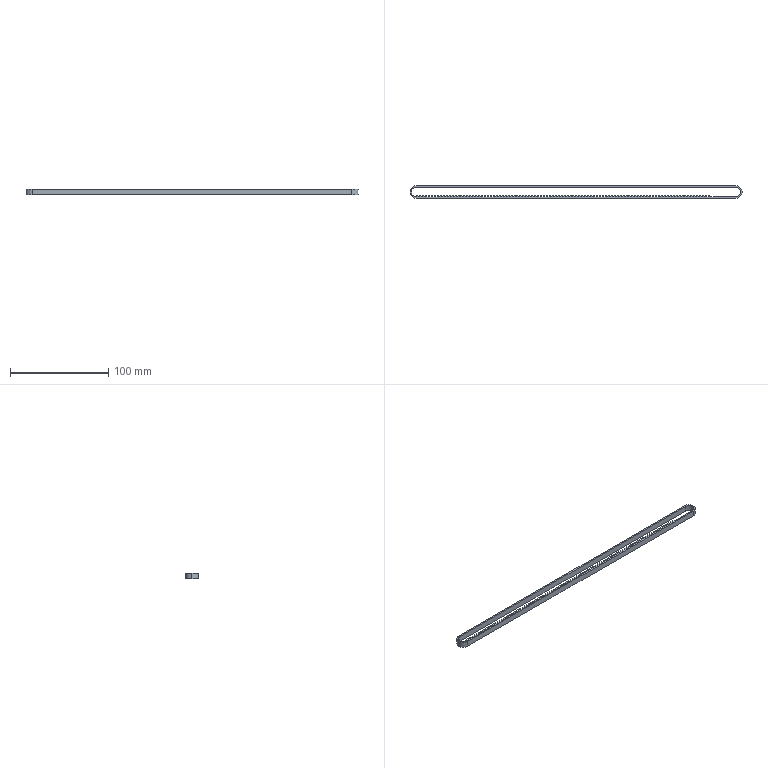Part | SolidWorks | features Extrusion 1, ICE 1, LPattern 1 | 1 solid | 411 faces | box 338 x 13 x 6 mm | volume 7437 mm3 | plane 405 | cylinder 6 | commonest cylinder face diameters 10 x3 13 x3